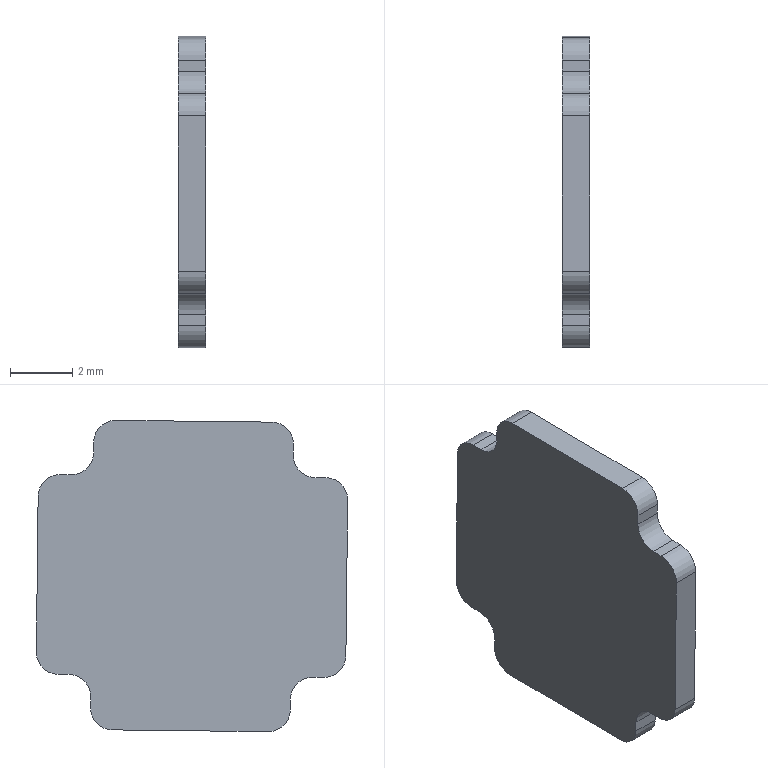Part | SolidWorks | features SplitBody 1 | 1 solid | 26 faces | box 0.88 x 9.983 x 9.983 mm | volume 75.431 mm3 | plane 14 | cylinder 12 | commonest cylinder face diameters 1.408 x12
STEP:
#1=CARTESIAN_POINT('',(584.115,440.454,-345.037));
#2=VERTEX_POINT('',#1);
#3=CARTESIAN_POINT('',(584.115,441.166,-345.733));
#4=VERTEX_POINT('',#3);
#5=CARTESIAN_POINT('',(584.115,441.158,-345.029));
#6=DIRECTION('',(1.,0.,0.));
#7=DIRECTION('',(0.,0.9999,0.01138));
#8=AXIS2_PLACEMENT_3D('',#5,#6,#7);
#9=CIRCLE('',#8,0.704);
#10=EDGE_CURVE('',#2,#4,#9,.T.);
#11=ORIENTED_EDGE('',*,*,#10,.T.);
#12=CARTESIAN_POINT('',(584.995,441.166,-345.733));
#13=VERTEX_POINT('',#12);
#14=CARTESIAN_POINT('',(584.995,441.166,-345.733));
#15=DIRECTION('',(-1.,0.,0.));
#16=VECTOR('',#15,1000.);
#17=LINE('',#14,#16);
#18=EDGE_CURVE('',#13,#4,#17,.T.);
#19=ORIENTED_EDGE('',*,*,#18,.F.);
#20=CARTESIAN_POINT('',(584.995,440.454,-345.037));
#21=VERTEX_POINT('',#20);
#22=CARTESIAN_POINT('',(584.995,441.158,-345.029));
#23=DIRECTION('',(1.,0.,0.));
#24=DIRECTION('',(0.,0.9999,0.01138));
#25=AXIS2_PLACEMENT_3D('',#22,#23,#24);
#26=CIRCLE('',#25,0.704);
#27=EDGE_CURVE('',#21,#13,#26,.T.);
#28=ORIENTED_EDGE('',*,*,#27,.F.);
#29=CARTESIAN_POINT('',(584.995,440.454,-345.037));
#30=DIRECTION('',(-1.,0.,0.));
#31=VECTOR('',#30,1000.);
#32=LINE('',#29,#31);
#33=EDGE_CURVE('',#21,#2,#32,.T.);
#34=ORIENTED_EDGE('',*,*,#33,.T.);
#35=EDGE_LOOP('',(#11,#19,#28,#34));
#36=FACE_OUTER_BOUND('',#35,.T.);
#37=CARTESIAN_POINT('',(584.995,441.158,-345.029));
#38=DIRECTION('',(-1.,0.,0.));
#39=DIRECTION('',(0.,-0.9999,-0.01138));
#40=AXIS2_PLACEMENT_3D('',#37,#38,#39);
#41=CYLINDRICAL_SURFACE('',#40,0.704);
#42=ADVANCED_FACE('',(#36),#41,.T.);
#43=CARTESIAN_POINT('',(584.115,441.518,-345.729));
#44=VERTEX_POINT('',#43);
#45=CARTESIAN_POINT('',(584.115,441.166,-345.733));
#46=DIRECTION('',(0.,0.9999,0.01138));
#47=VECTOR('',#46,1000.);
#48=LINE('',#45,#47);
#49=EDGE_CURVE('',#4,#44,#48,.T.);
#50=ORIENTED_EDGE('',*,*,#49,.T.);
#51=CARTESIAN_POINT('',(584.995,441.518,-345.729));
#52=VERTEX_POINT('',#51);
#53=CARTESIAN_POINT('',(584.995,441.518,-345.729));
#54=DIRECTION('',(-1.,0.,0.));
#55=VECTOR('',#54,1000.);
#56=LINE('',#53,#55);
#57=EDGE_CURVE('',#52,#44,#56,.T.);
#58=ORIENTED_EDGE('',*,*,#57,.F.);
#59=CARTESIAN_POINT('',(584.995,441.166,-345.733));
#60=DIRECTION('',(0.,0.9999,0.01138));
#61=VECTOR('',#60,1000.);
#62=LINE('',#59,#61);
#63=EDGE_CURVE('',#13,#52,#62,.T.);
#64=ORIENTED_EDGE('',*,*,#63,.F.);
#65=ORIENTED_EDGE('',*,*,#18,.T.);
#66=EDGE_LOOP('',(#50,#58,#64,#65));
#67=FACE_OUTER_BOUND('',#66,.T.);
#68=CARTESIAN_POINT('',(584.995,441.166,-345.733));
#69=DIRECTION('',(0.,-0.01138,0.9999));
#70=DIRECTION('',(1.,0.,0.));
#71=AXIS2_PLACEMENT_3D('',#68,#69,#70);
#72=PLANE('',#71);
#73=ADVANCED_FACE('',(#67),#72,.F.);
#74=CARTESIAN_POINT('',(584.115,442.23,-346.425));
#75=VERTEX_POINT('',#74);
#76=CARTESIAN_POINT('',(584.115,441.526,-346.433));
#77=DIRECTION('',(-1.,0.,0.));
#78=DIRECTION('',(0.,0.9999,0.01138));
#79=AXIS2_PLACEMENT_3D('',#76,#77,#78);
#80=CIRCLE('',#79,0.704);
#81=EDGE_CURVE('',#44,#75,#80,.T.);
#82=ORIENTED_EDGE('',*,*,#81,.T.);
#83=CARTESIAN_POINT('',(584.995,442.23,-346.425));
#84=VERTEX_POINT('',#83);
#85=CARTESIAN_POINT('',(584.995,442.23,-346.425));
#86=DIRECTION('',(-1.,0.,0.));
#87=VECTOR('',#86,1000.);
#88=LINE('',#85,#87);
#89=EDGE_CURVE('',#84,#75,#88,.T.);
#90=ORIENTED_EDGE('',*,*,#89,.F.);
#91=CARTESIAN_POINT('',(584.995,441.526,-346.433));
#92=DIRECTION('',(-1.,0.,0.));
#93=DIRECTION('',(0.,0.9999,0.01138));
#94=AXIS2_PLACEMENT_3D('',#91,#92,#93);
#95=CIRCLE('',#94,0.704);
#96=EDGE_CURVE('',#52,#84,#95,.T.);
#97=ORIENTED_EDGE('',*,*,#96,.F.);
#98=ORIENTED_EDGE('',*,*,#57,.T.);
#99=EDGE_LOOP('',(#82,#90,#97,#98));
#100=FACE_OUTER_BOUND('',#99,.T.);
#101=CARTESIAN_POINT('',(584.995,441.526,-346.433));
#102=DIRECTION('',(-1.,0.,0.));
#103=DIRECTION('',(0.,-0.9999,-0.01138));
#104=AXIS2_PLACEMENT_3D('',#101,#102,#103);
#105=CYLINDRICAL_SURFACE('',#104,0.704);
#106=ADVANCED_FACE('',(#100),#105,.F.);
#107=CARTESIAN_POINT('',(584.115,442.234,-346.777));
#108=VERTEX_POINT('',#107);
#109=CARTESIAN_POINT('',(584.115,442.23,-346.425));
#110=DIRECTION('',(0.,0.01138,-0.9999));
#111=VECTOR('',#110,1000.);
#112=LINE('',#109,#111);
#113=EDGE_CURVE('',#75,#108,#112,.T.);
#114=ORIENTED_EDGE('',*,*,#113,.T.);
#115=CARTESIAN_POINT('',(584.995,442.234,-346.777));
#116=VERTEX_POINT('',#115);
#117=CARTESIAN_POINT('',(584.995,442.234,-346.777));
#118=DIRECTION('',(-1.,0.,0.));
#119=VECTOR('',#118,1000.);
#120=LINE('',#117,#119);
#121=EDGE_CURVE('',#116,#108,#120,.T.);
#122=ORIENTED_EDGE('',*,*,#121,.F.);
#123=CARTESIAN_POINT('',(584.995,442.23,-346.425));
#124=DIRECTION('',(0.,0.01138,-0.9999));
#125=VECTOR('',#124,1000.);
#126=LINE('',#123,#125);
#127=EDGE_CURVE('',#84,#116,#126,.T.);
#128=ORIENTED_EDGE('',*,*,#127,.F.);
#129=ORIENTED_EDGE('',*,*,#89,.T.);
#130=EDGE_LOOP('',(#114,#122,#128,#129));
#131=FACE_OUTER_BOUND('',#130,.T.);
#132=CARTESIAN_POINT('',(584.995,442.23,-346.425));
#133=DIRECTION('',(0.,0.9999,0.01138));
#134=DIRECTION('',(-1.,0.,0.));
#135=AXIS2_PLACEMENT_3D('',#132,#133,#134);
#136=PLANE('',#135);
#137=ADVANCED_FACE('',(#131),#136,.F.);
#138=CARTESIAN_POINT('',(584.115,442.946,-347.473));
#139=VERTEX_POINT('',#138);
#140=CARTESIAN_POINT('',(584.115,442.938,-346.769));
#141=DIRECTION('',(1.,0.,0.));
#142=DIRECTION('',(0.,0.9999,0.01138));
#143=AXIS2_PLACEMENT_3D('',#140,#141,#142);
#144=CIRCLE('',#143,0.704);
#145=EDGE_CURVE('',#108,#139,#144,.T.);
#146=ORIENTED_EDGE('',*,*,#145,.T.);
#147=CARTESIAN_POINT('',(584.995,442.946,-347.473));
#148=VERTEX_POINT('',#147);
#149=CARTESIAN_POINT('',(584.995,442.946,-347.473));
#150=DIRECTION('',(-1.,0.,0.));
#151=VECTOR('',#150,1000.);
#152=LINE('',#149,#151);
#153=EDGE_CURVE('',#148,#139,#152,.T.);
#154=ORIENTED_EDGE('',*,*,#153,.F.);
#155=CARTESIAN_POINT('',(584.995,442.938,-346.769));
#156=DIRECTION('',(1.,0.,0.));
#157=DIRECTION('',(0.,0.9999,0.01138));
#158=AXIS2_PLACEMENT_3D('',#155,#156,#157);
#159=CIRCLE('',#158,0.704);
#160=EDGE_CURVE('',#116,#148,#159,.T.);
#161=ORIENTED_EDGE('',*,*,#160,.F.);
#162=ORIENTED_EDGE('',*,*,#121,.T.);
#163=EDGE_LOOP('',(#146,#154,#161,#162));
#164=FACE_OUTER_BOUND('',#163,.T.);
#165=CARTESIAN_POINT('',(584.995,442.938,-346.769));
#166=DIRECTION('',(-1.,0.,0.));
#167=DIRECTION('',(0.,-0.9999,-0.01138));
#168=AXIS2_PLACEMENT_3D('',#165,#166,#167);
#169=CYLINDRICAL_SURFACE('',#168,0.704);
#170=ADVANCED_FACE('',(#164),#169,.T.);
#171=CARTESIAN_POINT('',(584.115,447.944,-347.416));
#172=VERTEX_POINT('',#171);
#173=CARTESIAN_POINT('',(584.115,442.946,-347.473));
#174=DIRECTION('',(0.,0.9999,0.01138));
#175=VECTOR('',#174,1000.);
#176=LINE('',#173,#175);
#177=EDGE_CURVE('',#139,#172,#176,.T.);
#178=ORIENTED_EDGE('',*,*,#177,.T.);
#179=CARTESIAN_POINT('',(584.995,447.944,-347.416));
#180=VERTEX_POINT('',#179);
#181=CARTESIAN_POINT('',(584.995,447.944,-347.416));
#182=DIRECTION('',(-1.,0.,0.));
#183=VECTOR('',#182,1000.);
#184=LINE('',#181,#183);
#185=EDGE_CURVE('',#180,#172,#184,.T.);
#186=ORIENTED_EDGE('',*,*,#185,.F.);
#187=CARTESIAN_POINT('',(584.995,442.946,-347.473));
#188=DIRECTION('',(0.,0.9999,0.01138));
#189=VECTOR('',#188,1000.);
#190=LINE('',#187,#189);
#191=EDGE_CURVE('',#148,#180,#190,.T.);
#192=ORIENTED_EDGE('',*,*,#191,.F.);
#193=ORIENTED_EDGE('',*,*,#153,.T.);
#194=EDGE_LOOP('',(#178,#186,#192,#193));
#195=FACE_OUTER_BOUND('',#194,.T.);
#196=CARTESIAN_POINT('',(584.995,442.946,-347.473));
#197=DIRECTION('',(0.,-0.01138,0.9999));
#198=DIRECTION('',(1.,0.,0.));
#199=AXIS2_PLACEMENT_3D('',#196,#197,#198);
#200=PLANE('',#199);
#201=ADVANCED_FACE('',(#195),#200,.F.);
#202=CARTESIAN_POINT('',(584.115,448.64,-346.704));
#203=VERTEX_POINT('',#202);
#204=CARTESIAN_POINT('',(584.115,447.936,-346.712));
#205=DIRECTION('',(1.,0.,0.));
#206=DIRECTION('',(0.,0.9999,0.01138));
#207=AXIS2_PLACEMENT_3D('',#204,#205,#206);
#208=CIRCLE('',#207,0.704);
#209=EDGE_CURVE('',#172,#203,#208,.T.);
#210=ORIENTED_EDGE('',*,*,#209,.T.);
#211=CARTESIAN_POINT('',(584.995,448.64,-346.704));
#212=VERTEX_POINT('',#211);
#213=CARTESIAN_POINT('',(584.995,448.64,-346.704));
#214=DIRECTION('',(-1.,0.,0.));
#215=VECTOR('',#214,1000.);
#216=LINE('',#213,#215);
#217=EDGE_CURVE('',#212,#203,#216,.T.);
#218=ORIENTED_EDGE('',*,*,#217,.F.);
#219=CARTESIAN_POINT('',(584.995,447.936,-346.712));
#220=DIRECTION('',(1.,0.,0.));
#221=DIRECTION('',(0.,0.9999,0.01138));
#222=AXIS2_PLACEMENT_3D('',#219,#220,#221);
#223=CIRCLE('',#222,0.704);
#224=EDGE_CURVE('',#180,#212,#223,.T.);
#225=ORIENTED_EDGE('',*,*,#224,.F.);
#226=ORIENTED_EDGE('',*,*,#185,.T.);
#227=EDGE_LOOP('',(#210,#218,#225,#226));
#228=FACE_OUTER_BOUND('',#227,.T.);
#229=CARTESIAN_POINT('',(584.995,447.936,-346.712));
#230=DIRECTION('',(-1.,0.,0.));
#231=DIRECTION('',(0.,-0.9999,-0.01138));
#232=AXIS2_PLACEMENT_3D('',#229,#230,#231);
#233=CYLINDRICAL_SURFACE('',#232,0.704);
#234=ADVANCED_FACE('',(#228),#233,.T.);
#235=CARTESIAN_POINT('',(584.115,448.636,-346.352));
#236=VERTEX_POINT('',#235);
#237=CARTESIAN_POINT('',(584.115,448.64,-346.704));
#238=DIRECTION('',(0.,-0.01138,0.9999));
#239=VECTOR('',#238,1000.);
#240=LINE('',#237,#239);
#241=EDGE_CURVE('',#203,#236,#240,.T.);
#242=ORIENTED_EDGE('',*,*,#241,.T.);
#243=CARTESIAN_POINT('',(584.995,448.636,-346.352));
#244=VERTEX_POINT('',#243);
#245=CARTESIAN_POINT('',(584.995,448.636,-346.352));
#246=DIRECTION('',(-1.,0.,0.));
#247=VECTOR('',#246,1000.);
#248=LINE('',#245,#247);
#249=EDGE_CURVE('',#244,#236,#248,.T.);
#250=ORIENTED_EDGE('',*,*,#249,.F.);
#251=CARTESIAN_POINT('',(584.995,448.64,-346.704));
#252=DIRECTION('',(0.,-0.01138,0.9999));
#253=VECTOR('',#252,1000.);
#254=LINE('',#251,#253);
#255=EDGE_CURVE('',#212,#244,#254,.T.);
#256=ORIENTED_EDGE('',*,*,#255,.F.);
#257=ORIENTED_EDGE('',*,*,#217,.T.);
#258=EDGE_LOOP('',(#242,#250,#256,#257));
#259=FACE_OUTER_BOUND('',#258,.T.);
#260=CARTESIAN_POINT('',(584.995,448.64,-346.704));
#261=DIRECTION('',(0.,-0.9999,-0.01138));
#262=DIRECTION('',(1.,0.,0.));
#263=AXIS2_PLACEMENT_3D('',#260,#261,#262);
#264=PLANE('',#263);
#265=ADVANCED_FACE('',(#259),#264,.F.);
#266=CARTESIAN_POINT('',(584.115,449.331,-345.64));
#267=VERTEX_POINT('',#266);
#268=CARTESIAN_POINT('',(584.115,449.339,-346.344));
#269=DIRECTION('',(-1.,0.,0.));
#270=DIRECTION('',(0.,0.9999,0.01138));
#271=AXIS2_PLACEMENT_3D('',#268,#269,#270);
#272=CIRCLE('',#271,0.704);
#273=EDGE_CURVE('',#236,#267,#272,.T.);
#274=ORIENTED_EDGE('',*,*,#273,.T.);
#275=CARTESIAN_POINT('',(584.995,449.331,-345.64));
#276=VERTEX_POINT('',#275);
#277=CARTESIAN_POINT('',(584.995,449.331,-345.64));
#278=DIRECTION('',(-1.,0.,0.));
#279=VECTOR('',#278,1000.);
#280=LINE('',#277,#279);
#281=EDGE_CURVE('',#276,#267,#280,.T.);
#282=ORIENTED_EDGE('',*,*,#281,.F.);
#283=CARTESIAN_POINT('',(584.995,449.339,-346.344));
#284=DIRECTION('',(-1.,0.,0.));
#285=DIRECTION('',(0.,0.9999,0.01138));
#286=AXIS2_PLACEMENT_3D('',#283,#284,#285);
#287=CIRCLE('',#286,0.704);
#288=EDGE_CURVE('',#244,#276,#287,.T.);
#289=ORIENTED_EDGE('',*,*,#288,.F.);
#290=ORIENTED_EDGE('',*,*,#249,.T.);
#291=EDGE_LOOP('',(#274,#282,#289,#290));
#292=FACE_OUTER_BOUND('',#291,.T.);
#293=CARTESIAN_POINT('',(584.995,449.339,-346.344));
#294=DIRECTION('',(-1.,0.,0.));
#295=DIRECTION('',(0.,-0.9999,-0.01138));
#296=AXIS2_PLACEMENT_3D('',#293,#294,#295);
#297=CYLINDRICAL_SURFACE('',#296,0.704);
#298=ADVANCED_FACE('',(#292),#297,.F.);
#299=CARTESIAN_POINT('',(584.115,449.683,-345.636));
#300=VERTEX_POINT('',#299);
#301=CARTESIAN_POINT('',(584.115,449.331,-345.64));
#302=DIRECTION('',(0.,0.9999,0.01138));
#303=VECTOR('',#302,1000.);
#304=LINE('',#301,#303);
#305=EDGE_CURVE('',#267,#300,#304,.T.);
#306=ORIENTED_EDGE('',*,*,#305,.T.);
#307=CARTESIAN_POINT('',(584.995,449.683,-345.636));
#308=VERTEX_POINT('',#307);
#309=CARTESIAN_POINT('',(584.995,449.683,-345.636));
#310=DIRECTION('',(-1.,0.,0.));
#311=VECTOR('',#310,1000.);
#312=LINE('',#309,#311);
#313=EDGE_CURVE('',#308,#300,#312,.T.);
#314=ORIENTED_EDGE('',*,*,#313,.F.);
#315=CARTESIAN_POINT('',(584.995,449.331,-345.64));
#316=DIRECTION('',(0.,0.9999,0.01138));
#317=VECTOR('',#316,1000.);
#318=LINE('',#315,#317);
#319=EDGE_CURVE('',#276,#308,#318,.T.);
#320=ORIENTED_EDGE('',*,*,#319,.F.);
#321=ORIENTED_EDGE('',*,*,#281,.T.);
#322=EDGE_LOOP('',(#306,#314,#320,#321));
#323=FACE_OUTER_BOUND('',#322,.T.);
#324=CARTESIAN_POINT('',(584.995,449.331,-345.64));
#325=DIRECTION('',(0.,-0.01138,0.9999));
#326=DIRECTION('',(1.,0.,0.));
#327=AXIS2_PLACEMENT_3D('',#324,#325,#326);
#328=PLANE('',#327);
#329=ADVANCED_FACE('',(#323),#328,.F.);
#330=CARTESIAN_POINT('',(584.115,450.379,-344.924));
#331=VERTEX_POINT('',#330);
#332=CARTESIAN_POINT('',(584.115,449.675,-344.932));
#333=DIRECTION('',(1.,0.,0.));
#334=DIRECTION('',(0.,0.9999,0.01138));
#335=AXIS2_PLACEMENT_3D('',#332,#333,#334);
#336=CIRCLE('',#335,0.704);
#337=EDGE_CURVE('',#300,#331,#336,.T.);
#338=ORIENTED_EDGE('',*,*,#337,.T.);
#339=CARTESIAN_POINT('',(584.995,450.379,-344.924));
#340=VERTEX_POINT('',#339);
#341=CARTESIAN_POINT('',(584.995,450.379,-344.924));
#342=DIRECTION('',(-1.,0.,0.));
#343=VECTOR('',#342,1000.);
#344=LINE('',#341,#343);
#345=EDGE_CURVE('',#340,#331,#344,.T.);
#346=ORIENTED_EDGE('',*,*,#345,.F.);
#347=CARTESIAN_POINT('',(584.995,449.675,-344.932));
#348=DIRECTION('',(1.,0.,0.));
#349=DIRECTION('',(0.,0.9999,0.01138));
#350=AXIS2_PLACEMENT_3D('',#347,#348,#349);
#351=CIRCLE('',#350,0.704);
#352=EDGE_CURVE('',#308,#340,#351,.T.);
#353=ORIENTED_EDGE('',*,*,#352,.F.);
#354=ORIENTED_EDGE('',*,*,#313,.T.);
#355=EDGE_LOOP('',(#338,#346,#353,#354));
#356=FACE_OUTER_BOUND('',#355,.T.);
#357=CARTESIAN_POINT('',(584.995,449.675,-344.932));
#358=DIRECTION('',(-1.,0.,0.));
#359=DIRECTION('',(0.,-0.9999,-0.01138));
#360=AXIS2_PLACEMENT_3D('',#357,#358,#359);
#361=CYLINDRICAL_SURFACE('',#360,0.704);
#362=ADVANCED_FACE('',(#356),#361,.T.);
#363=CARTESIAN_POINT('',(584.115,450.323,-339.926));
#364=VERTEX_POINT('',#363);
#365=CARTESIAN_POINT('',(584.115,450.379,-344.924));
#366=DIRECTION('',(0.,-0.01138,0.9999));
#367=VECTOR('',#366,1000.);
#368=LINE('',#365,#367);
#369=EDGE_CURVE('',#331,#364,#368,.T.);
#370=ORIENTED_EDGE('',*,*,#369,.T.);
#371=CARTESIAN_POINT('',(584.995,450.323,-339.926));
#372=VERTEX_POINT('',#371);
#373=CARTESIAN_POINT('',(584.995,450.323,-339.926));
#374=DIRECTION('',(-1.,0.,0.));
#375=VECTOR('',#374,1000.);
#376=LINE('',#373,#375);
#377=EDGE_CURVE('',#372,#364,#376,.T.);
#378=ORIENTED_EDGE('',*,*,#377,.F.);
#379=CARTESIAN_POINT('',(584.995,450.379,-344.924));
#380=DIRECTION('',(0.,-0.01138,0.9999));
#381=VECTOR('',#380,1000.);
#382=LINE('',#379,#381);
#383=EDGE_CURVE('',#340,#372,#382,.T.);
#384=ORIENTED_EDGE('',*,*,#383,.F.);
#385=ORIENTED_EDGE('',*,*,#345,.T.);
#386=EDGE_LOOP('',(#370,#378,#384,#385));
#387=FACE_OUTER_BOUND('',#386,.T.);
#388=CARTESIAN_POINT('',(584.995,450.379,-344.924));
#389=DIRECTION('',(0.,-0.9999,-0.01138));
#390=DIRECTION('',(0.,0.01138,-0.9999));
#391=AXIS2_PLACEMENT_3D('',#388,#389,#390);
#392=PLANE('',#391);
#393=ADVANCED_FACE('',(#387),#392,.F.);
#394=CARTESIAN_POINT('',(584.115,449.611,-339.23));
#395=VERTEX_POINT('',#394);
#396=CARTESIAN_POINT('',(584.115,449.619,-339.934));
#397=DIRECTION('',(1.,0.,0.));
#398=DIRECTION('',(0.,0.9999,0.01138));
#399=AXIS2_PLACEMENT_3D('',#396,#397,#398);
#400=CIRCLE('',#399,0.704);
#401=EDGE_CURVE('',#364,#395,#400,.T.);
#402=ORIENTED_EDGE('',*,*,#401,.T.);
#403=CARTESIAN_POINT('',(584.995,449.611,-339.23));
#404=VERTEX_POINT('',#403);
#405=CARTESIAN_POINT('',(584.995,449.611,-339.23));
#406=DIRECTION('',(-1.,0.,0.));
#407=VECTOR('',#406,1000.);
#408=LINE('',#405,#407);
#409=EDGE_CURVE('',#404,#395,#408,.T.);
#410=ORIENTED_EDGE('',*,*,#409,.F.);
#411=CARTESIAN_POINT('',(584.995,449.619,-339.934));
#412=DIRECTION('',(1.,0.,0.));
#413=DIRECTION('',(0.,0.9999,0.01138));
#414=AXIS2_PLACEMENT_3D('',#411,#412,#413);
#415=CIRCLE('',#414,0.704);
#416=EDGE_CURVE('',#372,#404,#415,.T.);
#417=ORIENTED_EDGE('',*,*,#416,.F.);
#418=ORIENTED_EDGE('',*,*,#377,.T.);
#419=EDGE_LOOP('',(#402,#410,#417,#418));
#420=FACE_OUTER_BOUND('',#419,.T.);
#421=CARTESIAN_POINT('',(584.995,449.619,-339.934));
#422=DIRECTION('',(-1.,0.,0.));
#423=DIRECTION('',(0.,-0.9999,-0.01138));
#424=AXIS2_PLACEMENT_3D('',#421,#422,#423);
#425=CYLINDRICAL_SURFACE('',#424,0.704);
#426=ADVANCED_FACE('',(#420),#425,.T.);
#427=CARTESIAN_POINT('',(584.115,449.259,-339.234));
#428=VERTEX_POINT('',#427);
#429=CARTESIAN_POINT('',(584.115,449.611,-339.23));
#430=DIRECTION('',(0.,-0.9999,-0.01138));
#431=VECTOR('',#430,1000.);
#432=LINE('',#429,#431);
#433=EDGE_CURVE('',#395,#428,#432,.T.);
#434=ORIENTED_EDGE('',*,*,#433,.T.);
#435=CARTESIAN_POINT('',(584.995,449.259,-339.234));
#436=VERTEX_POINT('',#435);
#437=CARTESIAN_POINT('',(584.995,449.259,-339.234));
#438=DIRECTION('',(-1.,0.,0.));
#439=VECTOR('',#438,1000.);
#440=LINE('',#437,#439);
#441=EDGE_CURVE('',#436,#428,#440,.T.);
#442=ORIENTED_EDGE('',*,*,#441,.F.);
#443=CARTESIAN_POINT('',(584.995,449.611,-339.23));
#444=DIRECTION('',(0.,-0.9999,-0.01138));
#445=VECTOR('',#444,1000.);
#446=LINE('',#443,#445);
#447=EDGE_CURVE('',#404,#436,#446,.T.);
#448=ORIENTED_EDGE('',*,*,#447,.F.);
#449=ORIENTED_EDGE('',*,*,#409,.T.);
#450=EDGE_LOOP('',(#434,#442,#448,#449));
#451=FACE_OUTER_BOUND('',#450,.T.);
#452=CARTESIAN_POINT('',(584.995,449.611,-339.23));
#453=DIRECTION('',(0.,0.01138,-0.9999));
#454=DIRECTION('',(-1.,0.,0.));
#455=AXIS2_PLACEMENT_3D('',#452,#453,#454);
#456=PLANE('',#455);
#457=ADVANCED_FACE('',(#451),#456,.F.);
#458=CARTESIAN_POINT('',(584.115,448.547,-338.538));
#459=VERTEX_POINT('',#458);
#460=CARTESIAN_POINT('',(584.115,449.251,-338.53));
#461=DIRECTION('',(-1.,0.,0.));
#462=DIRECTION('',(0.,0.9999,0.01138));
#463=AXIS2_PLACEMENT_3D('',#460,#461,#462);
#464=CIRCLE('',#463,0.704);
#465=EDGE_CURVE('',#428,#459,#464,.T.);
#466=ORIENTED_EDGE('',*,*,#465,.T.);
#467=CARTESIAN_POINT('',(584.995,448.547,-338.538));
#468=VERTEX_POINT('',#467);
#469=CARTESIAN_POINT('',(584.995,448.547,-338.538));
#470=DIRECTION('',(-1.,0.,0.));
#471=VECTOR('',#470,1000.);
#472=LINE('',#469,#471);
#473=EDGE_CURVE('',#468,#459,#472,.T.);
#474=ORIENTED_EDGE('',*,*,#473,.F.);
#475=CARTESIAN_POINT('',(584.995,449.251,-338.53));
#476=DIRECTION('',(-1.,0.,0.));
#477=DIRECTION('',(0.,0.9999,0.01138));
#478=AXIS2_PLACEMENT_3D('',#475,#476,#477);
#479=CIRCLE('',#478,0.704);
#480=EDGE_CURVE('',#436,#468,#479,.T.);
#481=ORIENTED_EDGE('',*,*,#480,.F.);
#482=ORIENTED_EDGE('',*,*,#441,.T.);
#483=EDGE_LOOP('',(#466,#474,#481,#482));
#484=FACE_OUTER_BOUND('',#483,.T.);
#485=CARTESIAN_POINT('',(584.995,449.251,-338.53));
#486=DIRECTION('',(-1.,0.,0.));
#487=DIRECTION('',(0.,-0.9999,-0.01138));
#488=AXIS2_PLACEMENT_3D('',#485,#486,#487);
#489=CYLINDRICAL_SURFACE('',#488,0.704);
#490=ADVANCED_FACE('',(#484),#489,.F.);
#491=CARTESIAN_POINT('',(584.115,448.543,-338.186));
#492=VERTEX_POINT('',#491);
#493=CARTESIAN_POINT('',(584.115,448.547,-338.538));
#494=DIRECTION('',(0.,-0.01138,0.9999));
#495=VECTOR('',#494,1000.);
#496=LINE('',#493,#495);
#497=EDGE_CURVE('',#459,#492,#496,.T.);
#498=ORIENTED_EDGE('',*,*,#497,.T.);
#499=CARTESIAN_POINT('',(584.995,448.543,-338.186));
#500=VERTEX_POINT('',#499);
#501=CARTESIAN_POINT('',(584.995,448.543,-338.186));
#502=DIRECTION('',(-1.,0.,0.));
#503=VECTOR('',#502,1000.);
#504=LINE('',#501,#503);
#505=EDGE_CURVE('',#500,#492,#504,.T.);
#506=ORIENTED_EDGE('',*,*,#505,.F.);
#507=CARTESIAN_POINT('',(584.995,448.547,-338.538));
#508=DIRECTION('',(0.,-0.01138,0.9999));
#509=VECTOR('',#508,1000.);
#510=LINE('',#507,#509);
#511=EDGE_CURVE('',#468,#500,#510,.T.);
#512=ORIENTED_EDGE('',*,*,#511,.F.);
#513=ORIENTED_EDGE('',*,*,#473,.T.);
#514=EDGE_LOOP('',(#498,#506,#512,#513));
#515=FACE_OUTER_BOUND('',#514,.T.);
#516=CARTESIAN_POINT('',(584.995,448.547,-338.538));
#517=DIRECTION('',(0.,-0.9999,-0.01138));
#518=DIRECTION('',(1.,0.,0.));
#519=AXIS2_PLACEMENT_3D('',#516,#517,#518);
#520=PLANE('',#519);
#521=ADVANCED_FACE('',(#515),#520,.F.);
#522=CARTESIAN_POINT('',(584.115,447.831,-337.49));
#523=VERTEX_POINT('',#522);
#524=CARTESIAN_POINT('',(584.115,447.839,-338.194));
#525=DIRECTION('',(1.,0.,0.));
#526=DIRECTION('',(0.,0.9999,0.01138));
#527=AXIS2_PLACEMENT_3D('',#524,#525,#526);
#528=CIRCLE('',#527,0.704);
#529=EDGE_CURVE('',#492,#523,#528,.T.);
#530=ORIENTED_EDGE('',*,*,#529,.T.);
#531=CARTESIAN_POINT('',(584.995,447.831,-337.49));
#532=VERTEX_POINT('',#531);
#533=CARTESIAN_POINT('',(584.995,447.831,-337.49));
#534=DIRECTION('',(-1.,0.,0.));
#535=VECTOR('',#534,1000.);
#536=LINE('',#533,#535);
#537=EDGE_CURVE('',#532,#523,#536,.T.);
#538=ORIENTED_EDGE('',*,*,#537,.F.);
#539=CARTESIAN_POINT('',(584.995,447.839,-338.194));
#540=DIRECTION('',(1.,0.,0.));
#541=DIRECTION('',(0.,0.9999,0.01138));
#542=AXIS2_PLACEMENT_3D('',#539,#540,#541);
#543=CIRCLE('',#542,0.704);
#544=EDGE_CURVE('',#500,#532,#543,.T.);
#545=ORIENTED_EDGE('',*,*,#544,.F.);
#546=ORIENTED_EDGE('',*,*,#505,.T.);
#547=EDGE_LOOP('',(#530,#538,#545,#546));
#548=FACE_OUTER_BOUND('',#547,.T.);
#549=CARTESIAN_POINT('',(584.995,447.839,-338.194));
#550=DIRECTION('',(-1.,0.,0.));
#551=DIRECTION('',(0.,-0.9999,-0.01138));
#552=AXIS2_PLACEMENT_3D('',#549,#550,#551);
#553=CYLINDRICAL_SURFACE('',#552,0.704);
#554=ADVANCED_FACE('',(#548),#553,.T.);
#555=CARTESIAN_POINT('',(584.115,442.833,-337.547));
#556=VERTEX_POINT('',#555);
#557=CARTESIAN_POINT('',(584.115,447.831,-337.49));
#558=DIRECTION('',(0.,-0.9999,-0.01138));
#559=VECTOR('',#558,1000.);
#560=LINE('',#557,#559);
#561=EDGE_CURVE('',#523,#556,#560,.T.);
#562=ORIENTED_EDGE('',*,*,#561,.T.);
#563=CARTESIAN_POINT('',(584.995,442.833,-337.547));
#564=VERTEX_POINT('',#563);
#565=CARTESIAN_POINT('',(584.995,442.833,-337.547));
#566=DIRECTION('',(-1.,0.,0.));
#567=VECTOR('',#566,1000.);
#568=LINE('',#565,#567);
#569=EDGE_CURVE('',#564,#556,#568,.T.);
#570=ORIENTED_EDGE('',*,*,#569,.F.);
#571=CARTESIAN_POINT('',(584.995,447.831,-337.49));
#572=DIRECTION('',(0.,-0.9999,-0.01138));
#573=VECTOR('',#572,1000.);
#574=LINE('',#571,#573);
#575=EDGE_CURVE('',#532,#564,#574,.T.);
#576=ORIENTED_EDGE('',*,*,#575,.F.);
#577=ORIENTED_EDGE('',*,*,#537,.T.);
#578=EDGE_LOOP('',(#562,#570,#576,#577));
#579=FACE_OUTER_BOUND('',#578,.T.);
#580=CARTESIAN_POINT('',(584.995,447.831,-337.49));
#581=DIRECTION('',(0.,0.01138,-0.9999));
#582=DIRECTION('',(-1.,0.,0.));
#583=AXIS2_PLACEMENT_3D('',#580,#581,#582);
#584=PLANE('',#583);
#585=ADVANCED_FACE('',(#579),#584,.F.);
#586=CARTESIAN_POINT('',(584.115,442.137,-338.259));
#587=VERTEX_POINT('',#586);
#588=CARTESIAN_POINT('',(584.115,442.841,-338.251));
#589=DIRECTION('',(1.,0.,0.));
#590=DIRECTION('',(0.,0.9999,0.01138));
#591=AXIS2_PLACEMENT_3D('',#588,#589,#590);
#592=CIRCLE('',#591,0.704);
#593=EDGE_CURVE('',#556,#587,#592,.T.);
#594=ORIENTED_EDGE('',*,*,#593,.T.);
#595=CARTESIAN_POINT('',(584.995,442.137,-338.259));
#596=VERTEX_POINT('',#595);
#597=CARTESIAN_POINT('',(584.995,442.137,-338.259));
#598=DIRECTION('',(-1.,0.,0.));
#599=VECTOR('',#598,1000.);
#600=LINE('',#597,#599);
#601=EDGE_CURVE('',#596,#587,#600,.T.);
#602=ORIENTED_EDGE('',*,*,#601,.F.);
#603=CARTESIAN_POINT('',(584.995,442.841,-338.251));
#604=DIRECTION('',(1.,0.,0.));
#605=DIRECTION('',(0.,0.9999,0.01138));
#606=AXIS2_PLACEMENT_3D('',#603,#604,#605);
#607=CIRCLE('',#606,0.704);
#608=EDGE_CURVE('',#564,#596,#607,.T.);
#609=ORIENTED_EDGE('',*,*,#608,.F.);
#610=ORIENTED_EDGE('',*,*,#569,.T.);
#611=EDGE_LOOP('',(#594,#602,#609,#610));
#612=FACE_OUTER_BOUND('',#611,.T.);
#613=CARTESIAN_POINT('',(584.995,442.841,-338.251));
#614=DIRECTION('',(-1.,0.,0.));
#615=DIRECTION('',(0.,-0.9999,-0.01138));
#616=AXIS2_PLACEMENT_3D('',#613,#614,#615);
#617=CYLINDRICAL_SURFACE('',#616,0.704);
#618=ADVANCED_FACE('',(#612),#617,.T.);
#619=CARTESIAN_POINT('',(584.115,442.141,-338.611));
#620=VERTEX_POINT('',#619);
#621=CARTESIAN_POINT('',(584.115,442.137,-338.259));
#622=DIRECTION('',(0.,0.01138,-0.9999));
#623=VECTOR('',#622,1000.);
#624=LINE('',#621,#623);
#625=EDGE_CURVE('',#587,#620,#624,.T.);
#626=ORIENTED_EDGE('',*,*,#625,.T.);
#627=CARTESIAN_POINT('',(584.995,442.141,-338.611));
#628=VERTEX_POINT('',#627);
#629=CARTESIAN_POINT('',(584.995,442.141,-338.611));
#630=DIRECTION('',(-1.,0.,0.));
#631=VECTOR('',#630,1000.);
#632=LINE('',#629,#631);
#633=EDGE_CURVE('',#628,#620,#632,.T.);
#634=ORIENTED_EDGE('',*,*,#633,.F.);
#635=CARTESIAN_POINT('',(584.995,442.137,-338.259));
#636=DIRECTION('',(0.,0.01138,-0.9999));
#637=VECTOR('',#636,1000.);
#638=LINE('',#635,#637);
#639=EDGE_CURVE('',#596,#628,#638,.T.);
#640=ORIENTED_EDGE('',*,*,#639,.F.);
#641=ORIENTED_EDGE('',*,*,#601,.T.);
#642=EDGE_LOOP('',(#626,#634,#640,#641));
#643=FACE_OUTER_BOUND('',#642,.T.);
#644=CARTESIAN_POINT('',(584.995,442.137,-338.259));
#645=DIRECTION('',(0.,0.9999,0.01138));
#646=DIRECTION('',(-1.,0.,0.));
#647=AXIS2_PLACEMENT_3D('',#644,#645,#646);
#648=PLANE('',#647);
#649=ADVANCED_FACE('',(#643),#648,.F.);
#650=CARTESIAN_POINT('',(584.115,441.445,-339.323));
#651=VERTEX_POINT('',#650);
#652=CARTESIAN_POINT('',(584.115,441.437,-338.619));
#653=DIRECTION('',(-1.,0.,0.));
#654=DIRECTION('',(0.,0.9999,0.01138));
#655=AXIS2_PLACEMENT_3D('',#652,#653,#654);
#656=CIRCLE('',#655,0.704);
#657=EDGE_CURVE('',#620,#651,#656,.T.);
#658=ORIENTED_EDGE('',*,*,#657,.T.);
#659=CARTESIAN_POINT('',(584.995,441.445,-339.323));
#660=VERTEX_POINT('',#659);
#661=CARTESIAN_POINT('',(584.995,441.445,-339.323));
#662=DIRECTION('',(-1.,0.,0.));
#663=VECTOR('',#662,1000.);
#664=LINE('',#661,#663);
#665=EDGE_CURVE('',#660,#651,#664,.T.);
#666=ORIENTED_EDGE('',*,*,#665,.F.);
#667=CARTESIAN_POINT('',(584.995,441.437,-338.619));
#668=DIRECTION('',(-1.,0.,0.));
#669=DIRECTION('',(0.,0.9999,0.01138));
#670=AXIS2_PLACEMENT_3D('',#667,#668,#669);
#671=CIRCLE('',#670,0.704);
#672=EDGE_CURVE('',#628,#660,#671,.T.);
#673=ORIENTED_EDGE('',*,*,#672,.F.);
#674=ORIENTED_EDGE('',*,*,#633,.T.);
#675=EDGE_LOOP('',(#658,#666,#673,#674));
#676=FACE_OUTER_BOUND('',#675,.T.);
#677=CARTESIAN_POINT('',(584.995,441.437,-338.619));
#678=DIRECTION('',(-1.,0.,0.));
#679=DIRECTION('',(0.,-0.9999,-0.01138));
#680=AXIS2_PLACEMENT_3D('',#677,#678,#679);
#681=CYLINDRICAL_SURFACE('',#680,0.704);
#682=ADVANCED_FACE('',(#676),#681,.F.);
#683=CARTESIAN_POINT('',(584.115,441.093,-339.327));
#684=VERTEX_POINT('',#683);
#685=CARTESIAN_POINT('',(584.115,441.445,-339.323));
#686=DIRECTION('',(0.,-0.9999,-0.01138));
#687=VECTOR('',#686,1000.);
#688=LINE('',#685,#687);
#689=EDGE_CURVE('',#651,#684,#688,.T.);
#690=ORIENTED_EDGE('',*,*,#689,.T.);
#691=CARTESIAN_POINT('',(584.995,441.093,-339.327));
#692=VERTEX_POINT('',#691);
#693=CARTESIAN_POINT('',(584.995,441.093,-339.327));
#694=DIRECTION('',(-1.,0.,0.));
#695=VECTOR('',#694,1000.);
#696=LINE('',#693,#695);
#697=EDGE_CURVE('',#692,#684,#696,.T.);
#698=ORIENTED_EDGE('',*,*,#697,.F.);
#699=CARTESIAN_POINT('',(584.995,441.445,-339.323));
#700=DIRECTION('',(0.,-0.9999,-0.01138));
#701=VECTOR('',#700,1000.);
#702=LINE('',#699,#701);
#703=EDGE_CURVE('',#660,#692,#702,.T.);
#704=ORIENTED_EDGE('',*,*,#703,.F.);
#705=ORIENTED_EDGE('',*,*,#665,.T.);
#706=EDGE_LOOP('',(#690,#698,#704,#705));
#707=FACE_OUTER_BOUND('',#706,.T.);
#708=CARTESIAN_POINT('',(584.995,441.445,-339.323));
#709=DIRECTION('',(0.,0.01138,-0.9999));
#710=DIRECTION('',(-1.,0.,0.));
#711=AXIS2_PLACEMENT_3D('',#708,#709,#710);
#712=PLANE('',#711);
#713=ADVANCED_FACE('',(#707),#712,.F.);
#714=CARTESIAN_POINT('',(584.115,440.397,-340.039));
#715=VERTEX_POINT('',#714);
#716=CARTESIAN_POINT('',(584.115,441.101,-340.031));
#717=DIRECTION('',(1.,0.,0.));
#718=DIRECTION('',(0.,0.9999,0.01138));
#719=AXIS2_PLACEMENT_3D('',#716,#717,#718);
#720=CIRCLE('',#719,0.704);
#721=EDGE_CURVE('',#684,#715,#720,.T.);
#722=ORIENTED_EDGE('',*,*,#721,.T.);
#723=CARTESIAN_POINT('',(584.995,440.397,-340.039));
#724=VERTEX_POINT('',#723);
#725=CARTESIAN_POINT('',(584.995,440.397,-340.039));
#726=DIRECTION('',(-1.,0.,0.));
#727=VECTOR('',#726,1000.);
#728=LINE('',#725,#727);
#729=EDGE_CURVE('',#724,#715,#728,.T.);
#730=ORIENTED_EDGE('',*,*,#729,.F.);
#731=CARTESIAN_POINT('',(584.995,441.101,-340.031));
#732=DIRECTION('',(1.,0.,0.));
#733=DIRECTION('',(0.,0.9999,0.01138));
#734=AXIS2_PLACEMENT_3D('',#731,#732,#733);
#735=CIRCLE('',#734,0.704);
#736=EDGE_CURVE('',#692,#724,#735,.T.);
#737=ORIENTED_EDGE('',*,*,#736,.F.);
#738=ORIENTED_EDGE('',*,*,#697,.T.);
#739=EDGE_LOOP('',(#722,#730,#737,#738));
#740=FACE_OUTER_BOUND('',#739,.T.);
#741=CARTESIAN_POINT('',(584.995,441.101,-340.031));
#742=DIRECTION('',(-1.,0.,0.));
#743=DIRECTION('',(0.,-0.9999,-0.01138));
#744=AXIS2_PLACEMENT_3D('',#741,#742,#743);
#745=CYLINDRICAL_SURFACE('',#744,0.704);
#746=ADVANCED_FACE('',(#740),#745,.T.);
#747=CARTESIAN_POINT('',(584.115,440.397,-340.039));
#748=DIRECTION('',(0.,0.01138,-0.9999));
#749=VECTOR('',#748,1000.);
#750=LINE('',#747,#749);
#751=EDGE_CURVE('',#715,#2,#750,.T.);
#752=ORIENTED_EDGE('',*,*,#751,.T.);
#753=ORIENTED_EDGE('',*,*,#33,.F.);
#754=CARTESIAN_POINT('',(584.995,440.397,-340.039));
#755=DIRECTION('',(0.,0.01138,-0.9999));
#756=VECTOR('',#755,1000.);
#757=LINE('',#754,#756);
#758=EDGE_CURVE('',#724,#21,#757,.T.);
#759=ORIENTED_EDGE('',*,*,#758,.F.);
#760=ORIENTED_EDGE('',*,*,#729,.T.);
#761=EDGE_LOOP('',(#752,#753,#759,#760));
#762=FACE_OUTER_BOUND('',#761,.T.);
#763=CARTESIAN_POINT('',(584.995,440.397,-340.039));
#764=DIRECTION('',(0.,0.9999,0.01138));
#765=DIRECTION('',(-1.,0.,0.));
#766=AXIS2_PLACEMENT_3D('',#763,#764,#765);
#767=PLANE('',#766);
#768=ADVANCED_FACE('',(#762),#767,.F.);
#769=ORIENTED_EDGE('',*,*,#27,.T.);
#770=ORIENTED_EDGE('',*,*,#63,.T.);
#771=ORIENTED_EDGE('',*,*,#96,.T.);
#772=ORIENTED_EDGE('',*,*,#127,.T.);
#773=ORIENTED_EDGE('',*,*,#160,.T.);
#774=ORIENTED_EDGE('',*,*,#191,.T.);
#775=ORIENTED_EDGE('',*,*,#224,.T.);
#776=ORIENTED_EDGE('',*,*,#255,.T.);
#777=ORIENTED_EDGE('',*,*,#288,.T.);
#778=ORIENTED_EDGE('',*,*,#319,.T.);
#779=ORIENTED_EDGE('',*,*,#352,.T.);
#780=ORIENTED_EDGE('',*,*,#383,.T.);
#781=ORIENTED_EDGE('',*,*,#416,.T.);
#782=ORIENTED_EDGE('',*,*,#447,.T.);
#783=ORIENTED_EDGE('',*,*,#480,.T.);
#784=ORIENTED_EDGE('',*,*,#511,.T.);
#785=ORIENTED_EDGE('',*,*,#544,.T.);
#786=ORIENTED_EDGE('',*,*,#575,.T.);
#787=ORIENTED_EDGE('',*,*,#608,.T.);
#788=ORIENTED_EDGE('',*,*,#639,.T.);
#789=ORIENTED_EDGE('',*,*,#672,.T.);
#790=ORIENTED_EDGE('',*,*,#703,.T.);
#791=ORIENTED_EDGE('',*,*,#736,.T.);
#792=ORIENTED_EDGE('',*,*,#758,.T.);
#793=EDGE_LOOP('',(#769,#770,#771,#772,#773,#774,#775,#776,#777,#778,#779,#780,#781,#782,#783,#784,#785,#786,#787,#788,#789,#790,#791,#792));
#794=FACE_OUTER_BOUND('',#793,.T.);
#795=CARTESIAN_POINT('',(584.995,441.158,-345.029));
#796=DIRECTION('',(1.,0.,0.));
#797=DIRECTION('',(0.,0.9999,0.01138));
#798=AXIS2_PLACEMENT_3D('',#795,#796,#797);
#799=PLANE('',#798);
#800=ADVANCED_FACE('',(#794),#799,.T.);
#801=ORIENTED_EDGE('',*,*,#10,.F.);
#802=ORIENTED_EDGE('',*,*,#751,.F.);
#803=ORIENTED_EDGE('',*,*,#721,.F.);
#804=ORIENTED_EDGE('',*,*,#689,.F.);
#805=ORIENTED_EDGE('',*,*,#657,.F.);
#806=ORIENTED_EDGE('',*,*,#625,.F.);
#807=ORIENTED_EDGE('',*,*,#593,.F.);
#808=ORIENTED_EDGE('',*,*,#561,.F.);
#809=ORIENTED_EDGE('',*,*,#529,.F.);
#810=ORIENTED_EDGE('',*,*,#497,.F.);
#811=ORIENTED_EDGE('',*,*,#465,.F.);
#812=ORIENTED_EDGE('',*,*,#433,.F.);
#813=ORIENTED_EDGE('',*,*,#401,.F.);
#814=ORIENTED_EDGE('',*,*,#369,.F.);
#815=ORIENTED_EDGE('',*,*,#337,.F.);
#816=ORIENTED_EDGE('',*,*,#305,.F.);
#817=ORIENTED_EDGE('',*,*,#273,.F.);
#818=ORIENTED_EDGE('',*,*,#241,.F.);
#819=ORIENTED_EDGE('',*,*,#209,.F.);
#820=ORIENTED_EDGE('',*,*,#177,.F.);
#821=ORIENTED_EDGE('',*,*,#145,.F.);
#822=ORIENTED_EDGE('',*,*,#113,.F.);
#823=ORIENTED_EDGE('',*,*,#81,.F.);
#824=ORIENTED_EDGE('',*,*,#49,.F.);
#825=EDGE_LOOP('',(#801,#802,#803,#804,#805,#806,#807,#808,#809,#810,#811,#812,#813,#814,#815,#816,#817,#818,#819,#820,#821,#822,#823,#824));
#826=FACE_OUTER_BOUND('',#825,.T.);
#827=CARTESIAN_POINT('',(584.115,441.158,-345.029));
#828=DIRECTION('',(1.,0.,0.));
#829=DIRECTION('',(0.,0.9999,0.01138));
#830=AXIS2_PLACEMENT_3D('',#827,#828,#829);
#831=PLANE('',#830);
#832=ADVANCED_FACE('',(#826),#831,.F.);
#833=CLOSED_SHELL('',(#42,#73,#106,#137,#170,#201,#234,#265,#298,#329,#362,#393,#426,#457,#490,#521,#554,#585,#618,#649,#682,#713,#746,#768,#800,#832));
#834=MANIFOLD_SOLID_BREP('',#833);
#835=CARTESIAN_POINT('',(0.,0.,0.));
#836=DIRECTION('',(0.,0.,1.));
#837=DIRECTION('',(1.,0.,0.));
#838=AXIS2_PLACEMENT_3D('',#835,#836,#837);
#839=(LENGTH_UNIT()NAMED_UNIT(*)SI_UNIT(.MILLI.,.METRE.));
#840=UNCERTAINTY_MEASURE_WITH_UNIT(LENGTH_MEASURE(0.00001),#839,'','');
#841=(NAMED_UNIT(*)PLANE_ANGLE_UNIT()SI_UNIT($,.RADIAN.));
#842=(NAMED_UNIT(*)SI_UNIT($,.STERADIAN.)SOLID_ANGLE_UNIT());
#843=(GEOMETRIC_REPRESENTATION_CONTEXT(3)GLOBAL_UNCERTAINTY_ASSIGNED_CONTEXT((#840))GLOBAL_UNIT_ASSIGNED_CONTEXT((#839,#841,#842))REPRESENTATION_CONTEXT('',''));
#844=ADVANCED_BREP_SHAPE_REPRESENTATION('',(#834,#838),#843);